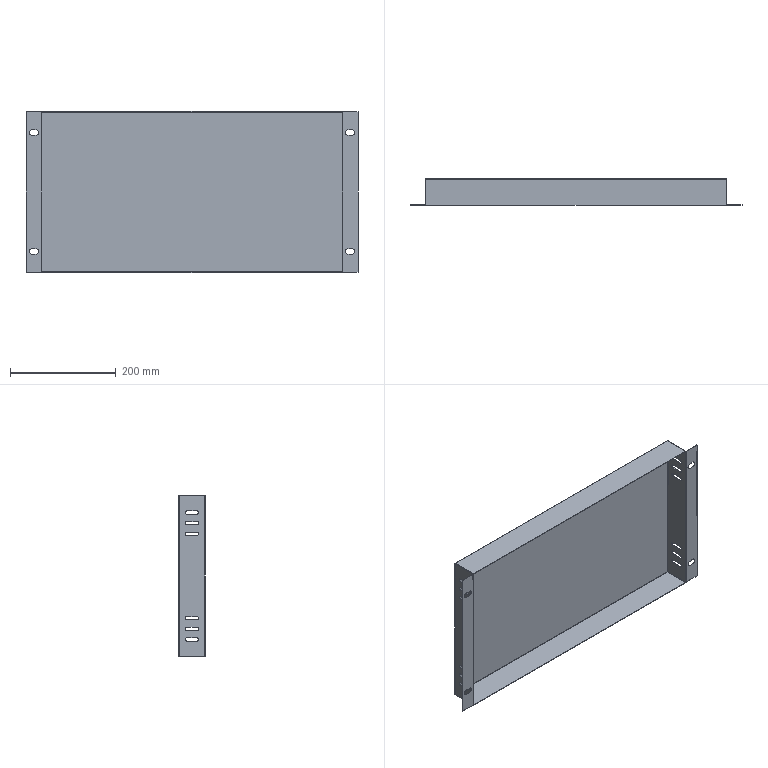Part | SolidWorks | features EdgeFlange 2, ICE 2, FlatPattern 1, SMBaseFlange 1, SheetMetal 1 | 1 solid | 130 faces | box 628 x 50 x 305 mm | volume 273586 mm3 | plane 66 | cylinder 56 | spline 8 | commonest cylinder face diameters 6 x36 10 x8 0.4 x6 2.4 x6